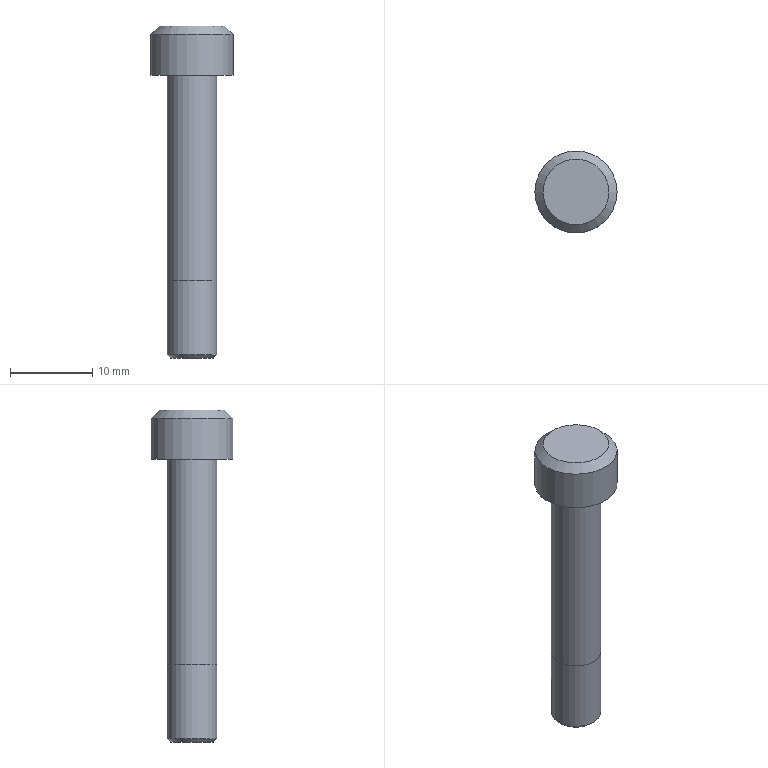Part | NX | features PG_666 2 | 1 solid | 11 faces | box 10 x 10 x 40.401 mm | volume 1207 mm3 | cylinder 4 | plane 4 | cone 3 | commonest cylinder face diameters 5.206 x2 6.007 x1 10 x1
STEP:
#1=CARTESIAN_POINT('',(2926.767,-936.298,814.716));
#2=VERTEX_POINT('',#1);
#3=CARTESIAN_POINT('',(2929.771,-936.298,814.716));
#4=DIRECTION('',(0.,0.,-1.));
#5=DIRECTION('',(-1.,0.,0.));
#6=AXIS2_PLACEMENT_3D('',#3,#4,#5);
#7=CIRCLE('',#6,3.003);
#8=EDGE_CURVE('',#2,#2,#7,.F.);
#9=ORIENTED_EDGE('',*,*,#8,.T.);
#10=EDGE_LOOP('',(#9));
#11=FACE_BOUND('',#10,.T.);
#12=CARTESIAN_POINT('',(2926.767,-936.298,848.716));
#13=VERTEX_POINT('',#12);
#14=CARTESIAN_POINT('',(2929.771,-936.298,848.716));
#15=DIRECTION('',(0.,0.,-1.));
#16=DIRECTION('',(-1.,0.,0.));
#17=AXIS2_PLACEMENT_3D('',#14,#15,#16);
#18=CIRCLE('',#17,3.003);
#19=EDGE_CURVE('',#13,#13,#18,.F.);
#20=ORIENTED_EDGE('',*,*,#19,.F.);
#21=EDGE_LOOP('',(#20));
#22=FACE_BOUND('',#21,.T.);
#23=CARTESIAN_POINT('',(2929.771,-936.298,808.716));
#24=DIRECTION('',(0.,0.,1.));
#25=DIRECTION('',(1.,0.,0.));
#26=AXIS2_PLACEMENT_3D('',#23,#24,#25);
#27=CYLINDRICAL_SURFACE('',#26,3.003);
#28=ADVANCED_FACE('',(#11,#22),#27,.T.);
#29=CARTESIAN_POINT('',(2933.771,-936.298,854.716));
#30=VERTEX_POINT('',#29);
#31=CARTESIAN_POINT('',(2929.771,-936.298,854.716));
#32=DIRECTION('',(0.,0.,1.));
#33=DIRECTION('',(1.,0.,0.));
#34=AXIS2_PLACEMENT_3D('',#31,#32,#33);
#35=CIRCLE('',#34,4.);
#36=EDGE_CURVE('',#30,#30,#35,.T.);
#37=ORIENTED_EDGE('',*,*,#36,.T.);
#38=EDGE_LOOP('',(#37));
#39=FACE_BOUND('',#38,.T.);
#40=CARTESIAN_POINT('',(2929.771,-936.298,854.716));
#41=DIRECTION('',(0.,0.,1.));
#42=DIRECTION('',(1.,0.,0.));
#43=AXIS2_PLACEMENT_3D('',#40,#41,#42);
#44=PLANE('',#43);
#45=ADVANCED_FACE('',(#39),#44,.T.);
#46=ORIENTED_EDGE('',*,*,#19,.T.);
#47=EDGE_LOOP('',(#46));
#48=FACE_BOUND('',#47,.T.);
#49=CARTESIAN_POINT('',(2934.771,-936.298,848.716));
#50=VERTEX_POINT('',#49);
#51=CARTESIAN_POINT('',(2929.771,-936.298,848.716));
#52=DIRECTION('',(0.,0.,1.));
#53=DIRECTION('',(1.,0.,0.));
#54=AXIS2_PLACEMENT_3D('',#51,#52,#53);
#55=CIRCLE('',#54,5.);
#56=EDGE_CURVE('',#50,#50,#55,.T.);
#57=ORIENTED_EDGE('',*,*,#56,.F.);
#58=EDGE_LOOP('',(#57));
#59=FACE_BOUND('',#58,.T.);
#60=CARTESIAN_POINT('',(2929.771,-936.298,848.716));
#61=DIRECTION('',(0.,0.,-1.));
#62=DIRECTION('',(-1.,0.,0.));
#63=AXIS2_PLACEMENT_3D('',#60,#61,#62);
#64=PLANE('',#63);
#65=ADVANCED_FACE('',(#48,#59),#64,.T.);
#66=CARTESIAN_POINT('',(2934.771,-936.298,853.716));
#67=VERTEX_POINT('',#66);
#68=CARTESIAN_POINT('',(2929.771,-936.298,853.716));
#69=DIRECTION('',(0.,0.,1.));
#70=DIRECTION('',(1.,0.,0.));
#71=AXIS2_PLACEMENT_3D('',#68,#69,#70);
#72=CIRCLE('',#71,5.);
#73=EDGE_CURVE('',#67,#67,#72,.F.);
#74=ORIENTED_EDGE('',*,*,#73,.T.);
#75=EDGE_LOOP('',(#74));
#76=FACE_BOUND('',#75,.T.);
#77=ORIENTED_EDGE('',*,*,#56,.T.);
#78=EDGE_LOOP('',(#77));
#79=FACE_BOUND('',#78,.T.);
#80=CARTESIAN_POINT('',(2929.771,-936.298,848.716));
#81=DIRECTION('',(0.,0.,1.));
#82=DIRECTION('',(1.,0.,0.));
#83=AXIS2_PLACEMENT_3D('',#80,#81,#82);
#84=CYLINDRICAL_SURFACE('',#83,5.);
#85=ADVANCED_FACE('',(#76,#79),#84,.T.);
#86=CARTESIAN_POINT('',(2932.374,-936.298,814.316));
#87=VERTEX_POINT('',#86);
#88=CARTESIAN_POINT('',(2929.771,-936.298,814.316));
#89=DIRECTION('',(0.,0.,1.));
#90=DIRECTION('',(1.,0.,0.));
#91=AXIS2_PLACEMENT_3D('',#88,#89,#90);
#92=CIRCLE('',#91,2.603);
#93=EDGE_CURVE('',#87,#87,#92,.F.);
#94=ORIENTED_EDGE('',*,*,#93,.F.);
#95=EDGE_LOOP('',(#94));
#96=FACE_BOUND('',#95,.T.);
#97=ORIENTED_EDGE('',*,*,#8,.F.);
#98=EDGE_LOOP('',(#97));
#99=FACE_BOUND('',#98,.T.);
#100=CARTESIAN_POINT('',(2929.771,-936.298,814.716));
#101=DIRECTION('',(0.,0.,1.));
#102=DIRECTION('',(1.,0.,0.));
#103=AXIS2_PLACEMENT_3D('',#100,#101,#102);
#104=CONICAL_SURFACE('',#103,3.003,0.7854);
#105=ADVANCED_FACE('',(#96,#99),#104,.T.);
#106=ORIENTED_EDGE('',*,*,#36,.F.);
#107=EDGE_LOOP('',(#106));
#108=FACE_BOUND('',#107,.T.);
#109=ORIENTED_EDGE('',*,*,#73,.F.);
#110=EDGE_LOOP('',(#109));
#111=FACE_BOUND('',#110,.T.);
#112=CARTESIAN_POINT('',(2929.771,-936.298,853.716));
#113=DIRECTION('',(0.,0.,-1.));
#114=DIRECTION('',(-1.,0.,0.));
#115=AXIS2_PLACEMENT_3D('',#112,#113,#114);
#116=CONICAL_SURFACE('',#115,5.,0.7854);
#117=ADVANCED_FACE('',(#108,#111),#116,.T.);
#118=CARTESIAN_POINT('',(2932.374,-936.298,823.716));
#119=VERTEX_POINT('',#118);
#120=CARTESIAN_POINT('',(2929.771,-936.298,823.716));
#121=DIRECTION('',(0.,0.,1.));
#122=DIRECTION('',(1.,0.,0.));
#123=AXIS2_PLACEMENT_3D('',#120,#121,#122);
#124=CIRCLE('',#123,2.603);
#125=EDGE_CURVE('',#119,#119,#124,.T.);
#126=ORIENTED_EDGE('',*,*,#125,.F.);
#127=EDGE_LOOP('',(#126));
#128=FACE_BOUND('',#127,.T.);
#129=CARTESIAN_POINT('',(2932.374,-936.298,824.716));
#130=VERTEX_POINT('',#129);
#131=CARTESIAN_POINT('',(2929.771,-936.298,824.716));
#132=DIRECTION('',(0.,0.,1.));
#133=DIRECTION('',(1.,0.,0.));
#134=AXIS2_PLACEMENT_3D('',#131,#132,#133);
#135=CIRCLE('',#134,2.603);
#136=EDGE_CURVE('',#130,#130,#135,.T.);
#137=ORIENTED_EDGE('',*,*,#136,.T.);
#138=EDGE_LOOP('',(#137));
#139=FACE_BOUND('',#138,.T.);
#140=CARTESIAN_POINT('',(2929.771,-936.298,823.716));
#141=DIRECTION('',(0.,0.,-1.));
#142=DIRECTION('',(1.,0.,0.));
#143=AXIS2_PLACEMENT_3D('',#140,#141,#142);
#144=CYLINDRICAL_SURFACE('',#143,2.603);
#145=ADVANCED_FACE('',(#128,#139),#144,.F.);
#146=ORIENTED_EDGE('',*,*,#136,.F.);
#147=EDGE_LOOP('',(#146));
#148=FACE_BOUND('',#147,.T.);
#149=CARTESIAN_POINT('',(2929.771,-936.298,824.716));
#150=DIRECTION('',(0.,0.,1.));
#151=DIRECTION('',(1.,0.,0.));
#152=AXIS2_PLACEMENT_3D('',#149,#150,#151);
#153=PLANE('',#152);
#154=ADVANCED_FACE('',(#148),#153,.F.);
#155=ORIENTED_EDGE('',*,*,#125,.T.);
#156=EDGE_LOOP('',(#155));
#157=FACE_BOUND('',#156,.T.);
#158=CARTESIAN_POINT('',(2932.771,-936.298,823.716));
#159=VERTEX_POINT('',#158);
#160=CARTESIAN_POINT('',(2929.771,-936.298,823.716));
#161=DIRECTION('',(0.,0.,-1.));
#162=DIRECTION('',(1.,0.,0.));
#163=AXIS2_PLACEMENT_3D('',#160,#161,#162);
#164=CIRCLE('',#163,3.);
#165=EDGE_CURVE('',#159,#159,#164,.F.);
#166=ORIENTED_EDGE('',*,*,#165,.F.);
#167=EDGE_LOOP('',(#166));
#168=FACE_BOUND('',#167,.T.);
#169=CARTESIAN_POINT('',(2929.771,-936.298,823.716));
#170=DIRECTION('',(0.,0.,1.));
#171=DIRECTION('',(1.,0.,0.));
#172=AXIS2_PLACEMENT_3D('',#169,#170,#171);
#173=PLANE('',#172);
#174=ADVANCED_FACE('',(#157,#168),#173,.F.);
#175=CARTESIAN_POINT('',(2932.374,-936.298,823.319));
#176=VERTEX_POINT('',#175);
#177=CARTESIAN_POINT('',(2929.771,-936.298,823.319));
#178=DIRECTION('',(0.,0.,1.));
#179=DIRECTION('',(1.,0.,0.));
#180=AXIS2_PLACEMENT_3D('',#177,#178,#179);
#181=CIRCLE('',#180,2.603);
#182=EDGE_CURVE('',#176,#176,#181,.F.);
#183=ORIENTED_EDGE('',*,*,#182,.T.);
#184=EDGE_LOOP('',(#183));
#185=FACE_BOUND('',#184,.T.);
#186=ORIENTED_EDGE('',*,*,#165,.T.);
#187=EDGE_LOOP('',(#186));
#188=FACE_BOUND('',#187,.T.);
#189=CARTESIAN_POINT('',(2929.771,-936.298,823.716));
#190=DIRECTION('',(0.,0.,1.));
#191=DIRECTION('',(1.,0.,0.));
#192=AXIS2_PLACEMENT_3D('',#189,#190,#191);
#193=CONICAL_SURFACE('',#192,3.,0.7854);
#194=ADVANCED_FACE('',(#185,#188),#193,.F.);
#195=ORIENTED_EDGE('',*,*,#93,.T.);
#196=EDGE_LOOP('',(#195));
#197=FACE_BOUND('',#196,.T.);
#198=ORIENTED_EDGE('',*,*,#182,.F.);
#199=EDGE_LOOP('',(#198));
#200=FACE_BOUND('',#199,.T.);
#201=CARTESIAN_POINT('',(2929.771,-936.298,823.716));
#202=DIRECTION('',(0.,0.,-1.));
#203=DIRECTION('',(1.,0.,0.));
#204=AXIS2_PLACEMENT_3D('',#201,#202,#203);
#205=CYLINDRICAL_SURFACE('',#204,2.603);
#206=ADVANCED_FACE('',(#197,#200),#205,.F.);
#207=CLOSED_SHELL('',(#28,#45,#65,#85,#105,#117,#145,#154,#174,#194,#206));
#208=MANIFOLD_SOLID_BREP('',#207);
#209=(LENGTH_UNIT()NAMED_UNIT(*)SI_UNIT(.MILLI.,.METRE.));
#210=UNCERTAINTY_MEASURE_WITH_UNIT(LENGTH_MEASURE(0.00001),#209,'','');
#211=(NAMED_UNIT(*)PLANE_ANGLE_UNIT()SI_UNIT($,.RADIAN.));
#212=(NAMED_UNIT(*)SI_UNIT($,.STERADIAN.)SOLID_ANGLE_UNIT());
#213=(GEOMETRIC_REPRESENTATION_CONTEXT(3)GLOBAL_UNCERTAINTY_ASSIGNED_CONTEXT((#210))GLOBAL_UNIT_ASSIGNED_CONTEXT((#209,#211,#212))REPRESENTATION_CONTEXT('',''));
#214=ADVANCED_BREP_SHAPE_REPRESENTATION('',(#208),#213);